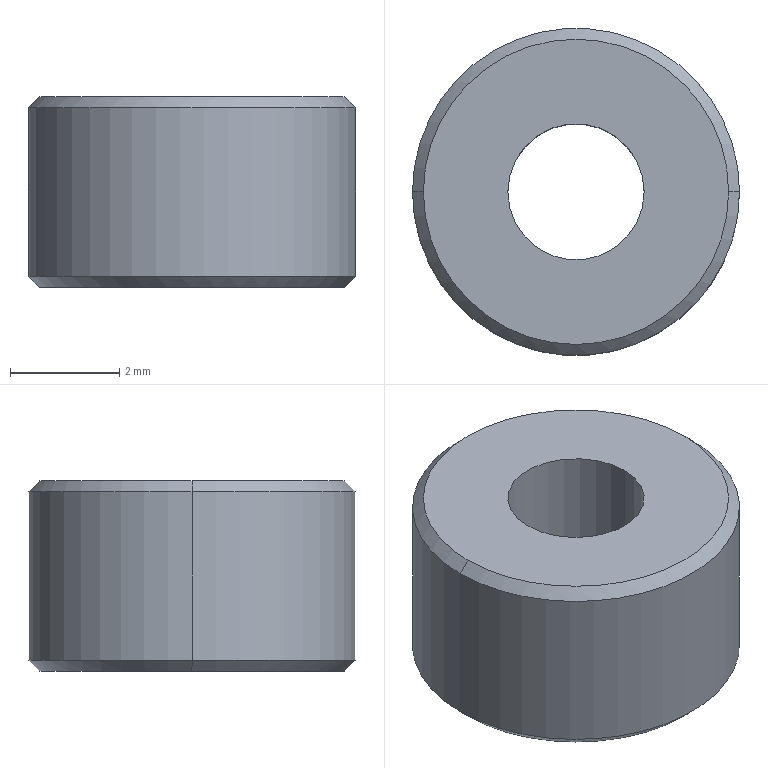Part | SolidWorks | features Chamfer 1, Extrusion 1, HoleWzd 1 | 1 solid | 10 faces | box 6 x 6 x 3.5 mm | volume 81.042 mm3 | cone 4 | cylinder 4 | plane 2 | commonest cylinder face diameters 2.5 x2 6 x2
STEP:
#1=CARTESIAN_POINT('',(2.8,0.,3.5));
#2=VERTEX_POINT('',#1);
#3=CARTESIAN_POINT('',(-2.8,0.,3.5));
#4=VERTEX_POINT('',#3);
#5=CARTESIAN_POINT('',(0.,0.,3.5));
#6=DIRECTION('',(0.,0.,1.));
#7=DIRECTION('',(1.,0.,0.));
#8=AXIS2_PLACEMENT_3D('',#5,#6,#7);
#9=CIRCLE('',#8,2.8);
#10=EDGE_CURVE('',#2,#4,#9,.T.);
#11=ORIENTED_EDGE('',*,*,#10,.F.);
#12=CARTESIAN_POINT('',(3.,0.,3.3));
#13=VERTEX_POINT('',#12);
#14=CARTESIAN_POINT('',(2.8,0.,3.5));
#15=DIRECTION('',(0.7071,0.,-0.7071));
#16=VECTOR('',#15,1000.);
#17=LINE('',#14,#16);
#18=EDGE_CURVE('',#2,#13,#17,.T.);
#19=ORIENTED_EDGE('',*,*,#18,.T.);
#20=CARTESIAN_POINT('',(-3.,0.,3.3));
#21=VERTEX_POINT('',#20);
#22=CARTESIAN_POINT('',(0.,0.,3.3));
#23=DIRECTION('',(0.,0.,-1.));
#24=DIRECTION('',(1.,0.,0.));
#25=AXIS2_PLACEMENT_3D('',#22,#23,#24);
#26=CIRCLE('',#25,3.);
#27=EDGE_CURVE('',#21,#13,#26,.T.);
#28=ORIENTED_EDGE('',*,*,#27,.F.);
#29=CARTESIAN_POINT('',(-2.8,0.,3.5));
#30=DIRECTION('',(-0.7071,0.,-0.7071));
#31=VECTOR('',#30,1000.);
#32=LINE('',#29,#31);
#33=EDGE_CURVE('',#4,#21,#32,.T.);
#34=ORIENTED_EDGE('',*,*,#33,.F.);
#35=EDGE_LOOP('',(#11,#19,#28,#34));
#36=FACE_OUTER_BOUND('',#35,.T.);
#37=CARTESIAN_POINT('',(0.,0.,3.5));
#38=DIRECTION('',(0.,0.,-1.));
#39=DIRECTION('',(-1.,0.,0.));
#40=AXIS2_PLACEMENT_3D('',#37,#38,#39);
#41=CONICAL_SURFACE('',#40,2.8,0.7854);
#42=ADVANCED_FACE('',(#36),#41,.T.);
#43=CARTESIAN_POINT('',(-2.8,0.,0.));
#44=VERTEX_POINT('',#43);
#45=CARTESIAN_POINT('',(2.8,0.,0.));
#46=VERTEX_POINT('',#45);
#47=CARTESIAN_POINT('',(0.,0.,0.));
#48=DIRECTION('',(0.,0.,-1.));
#49=DIRECTION('',(1.,0.,0.));
#50=AXIS2_PLACEMENT_3D('',#47,#48,#49);
#51=CIRCLE('',#50,2.8);
#52=EDGE_CURVE('',#44,#46,#51,.T.);
#53=ORIENTED_EDGE('',*,*,#52,.F.);
#54=CARTESIAN_POINT('',(-3.,0.,0.2));
#55=VERTEX_POINT('',#54);
#56=CARTESIAN_POINT('',(-3.,0.,0.2));
#57=DIRECTION('',(-0.7071,0.,0.7071));
#58=VECTOR('',#57,1000.);
#59=LINE('',#56,#58);
#60=EDGE_CURVE('',#44,#55,#59,.T.);
#61=ORIENTED_EDGE('',*,*,#60,.T.);
#62=CARTESIAN_POINT('',(3.,0.,0.2));
#63=VERTEX_POINT('',#62);
#64=CARTESIAN_POINT('',(0.,0.,0.2));
#65=DIRECTION('',(0.,0.,1.));
#66=DIRECTION('',(1.,0.,0.));
#67=AXIS2_PLACEMENT_3D('',#64,#65,#66);
#68=CIRCLE('',#67,3.);
#69=EDGE_CURVE('',#63,#55,#68,.T.);
#70=ORIENTED_EDGE('',*,*,#69,.F.);
#71=CARTESIAN_POINT('',(3.,0.,0.2));
#72=DIRECTION('',(0.7071,0.,0.7071));
#73=VECTOR('',#72,1000.);
#74=LINE('',#71,#73);
#75=EDGE_CURVE('',#46,#63,#74,.T.);
#76=ORIENTED_EDGE('',*,*,#75,.F.);
#77=EDGE_LOOP('',(#53,#61,#70,#76));
#78=FACE_OUTER_BOUND('',#77,.T.);
#79=CARTESIAN_POINT('',(0.,0.,0.2));
#80=DIRECTION('',(0.,0.,1.));
#81=DIRECTION('',(1.,0.,0.));
#82=AXIS2_PLACEMENT_3D('',#79,#80,#81);
#83=CONICAL_SURFACE('',#82,3.,0.7854);
#84=ADVANCED_FACE('',(#78),#83,.T.);
#85=CARTESIAN_POINT('',(-1.25,0.,3.5));
#86=VERTEX_POINT('',#85);
#87=CARTESIAN_POINT('',(1.25,0.,3.5));
#88=VERTEX_POINT('',#87);
#89=CARTESIAN_POINT('',(0.,0.,3.5));
#90=DIRECTION('',(0.,0.,1.));
#91=DIRECTION('',(1.,0.,0.));
#92=AXIS2_PLACEMENT_3D('',#89,#90,#91);
#93=CIRCLE('',#92,1.25);
#94=EDGE_CURVE('',#86,#88,#93,.T.);
#95=ORIENTED_EDGE('',*,*,#94,.T.);
#96=CARTESIAN_POINT('',(1.25,0.,0.));
#97=VERTEX_POINT('',#96);
#98=CARTESIAN_POINT('',(1.25,0.,0.));
#99=DIRECTION('',(0.,0.,-1.));
#100=VECTOR('',#99,1000.);
#101=LINE('',#98,#100);
#102=EDGE_CURVE('',#88,#97,#101,.T.);
#103=ORIENTED_EDGE('',*,*,#102,.T.);
#104=CARTESIAN_POINT('',(-1.25,0.,0.));
#105=VERTEX_POINT('',#104);
#106=CARTESIAN_POINT('',(0.,0.,0.));
#107=DIRECTION('',(0.,0.,-1.));
#108=DIRECTION('',(-1.,0.,0.));
#109=AXIS2_PLACEMENT_3D('',#106,#107,#108);
#110=CIRCLE('',#109,1.25);
#111=EDGE_CURVE('',#97,#105,#110,.T.);
#112=ORIENTED_EDGE('',*,*,#111,.T.);
#113=CARTESIAN_POINT('',(-1.25,0.,0.));
#114=DIRECTION('',(0.,0.,-1.));
#115=VECTOR('',#114,1000.);
#116=LINE('',#113,#115);
#117=EDGE_CURVE('',#86,#105,#116,.T.);
#118=ORIENTED_EDGE('',*,*,#117,.F.);
#119=EDGE_LOOP('',(#95,#103,#112,#118));
#120=FACE_OUTER_BOUND('',#119,.T.);
#121=CARTESIAN_POINT('',(0.,0.,0.));
#122=DIRECTION('',(0.,0.,-1.));
#123=DIRECTION('',(-1.,0.,0.));
#124=AXIS2_PLACEMENT_3D('',#121,#122,#123);
#125=CYLINDRICAL_SURFACE('',#124,1.25);
#126=ADVANCED_FACE('',(#120),#125,.F.);
#127=ORIENTED_EDGE('',*,*,#27,.T.);
#128=CARTESIAN_POINT('',(3.,0.,3.5));
#129=DIRECTION('',(0.,0.,-1.));
#130=VECTOR('',#129,1000.);
#131=LINE('',#128,#130);
#132=EDGE_CURVE('',#13,#63,#131,.T.);
#133=ORIENTED_EDGE('',*,*,#132,.T.);
#134=ORIENTED_EDGE('',*,*,#69,.T.);
#135=CARTESIAN_POINT('',(-3.,0.,3.5));
#136=DIRECTION('',(0.,0.,-1.));
#137=VECTOR('',#136,1000.);
#138=LINE('',#135,#137);
#139=EDGE_CURVE('',#21,#55,#138,.T.);
#140=ORIENTED_EDGE('',*,*,#139,.F.);
#141=EDGE_LOOP('',(#127,#133,#134,#140));
#142=FACE_OUTER_BOUND('',#141,.T.);
#143=CARTESIAN_POINT('',(0.,0.,3.5));
#144=DIRECTION('',(0.,0.,-1.));
#145=DIRECTION('',(-1.,0.,0.));
#146=AXIS2_PLACEMENT_3D('',#143,#144,#145);
#147=CYLINDRICAL_SURFACE('',#146,3.);
#148=ADVANCED_FACE('',(#142),#147,.T.);
#149=ORIENTED_EDGE('',*,*,#132,.F.);
#150=CARTESIAN_POINT('',(0.,0.,3.3));
#151=DIRECTION('',(0.,0.,-1.));
#152=DIRECTION('',(1.,0.,0.));
#153=AXIS2_PLACEMENT_3D('',#150,#151,#152);
#154=CIRCLE('',#153,3.);
#155=EDGE_CURVE('',#13,#21,#154,.T.);
#156=ORIENTED_EDGE('',*,*,#155,.T.);
#157=ORIENTED_EDGE('',*,*,#139,.T.);
#158=CARTESIAN_POINT('',(0.,0.,0.2));
#159=DIRECTION('',(0.,0.,1.));
#160=DIRECTION('',(1.,0.,0.));
#161=AXIS2_PLACEMENT_3D('',#158,#159,#160);
#162=CIRCLE('',#161,3.);
#163=EDGE_CURVE('',#55,#63,#162,.T.);
#164=ORIENTED_EDGE('',*,*,#163,.T.);
#165=EDGE_LOOP('',(#149,#156,#157,#164));
#166=FACE_OUTER_BOUND('',#165,.T.);
#167=CARTESIAN_POINT('',(0.,0.,3.5));
#168=DIRECTION('',(0.,0.,-1.));
#169=DIRECTION('',(-1.,0.,0.));
#170=AXIS2_PLACEMENT_3D('',#167,#168,#169);
#171=CYLINDRICAL_SURFACE('',#170,3.);
#172=ADVANCED_FACE('',(#166),#171,.T.);
#173=CARTESIAN_POINT('',(0.,0.,3.5));
#174=DIRECTION('',(0.,0.,1.));
#175=DIRECTION('',(1.,0.,0.));
#176=AXIS2_PLACEMENT_3D('',#173,#174,#175);
#177=CIRCLE('',#176,2.8);
#178=EDGE_CURVE('',#4,#2,#177,.T.);
#179=ORIENTED_EDGE('',*,*,#178,.T.);
#180=ORIENTED_EDGE('',*,*,#10,.T.);
#181=EDGE_LOOP('',(#179,#180));
#182=FACE_OUTER_BOUND('',#181,.T.);
#183=ORIENTED_EDGE('',*,*,#94,.F.);
#184=CARTESIAN_POINT('',(0.,0.,3.5));
#185=DIRECTION('',(0.,0.,1.));
#186=DIRECTION('',(1.,0.,0.));
#187=AXIS2_PLACEMENT_3D('',#184,#185,#186);
#188=CIRCLE('',#187,1.25);
#189=EDGE_CURVE('',#88,#86,#188,.T.);
#190=ORIENTED_EDGE('',*,*,#189,.F.);
#191=EDGE_LOOP('',(#183,#190));
#192=FACE_BOUND('',#191,.T.);
#193=CARTESIAN_POINT('',(0.,0.,3.5));
#194=DIRECTION('',(0.,0.,1.));
#195=DIRECTION('',(1.,0.,0.));
#196=AXIS2_PLACEMENT_3D('',#193,#194,#195);
#197=PLANE('',#196);
#198=ADVANCED_FACE('',(#182,#192),#197,.T.);
#199=CARTESIAN_POINT('',(0.,0.,0.));
#200=DIRECTION('',(0.,0.,-1.));
#201=DIRECTION('',(1.,0.,0.));
#202=AXIS2_PLACEMENT_3D('',#199,#200,#201);
#203=CIRCLE('',#202,2.8);
#204=EDGE_CURVE('',#46,#44,#203,.T.);
#205=ORIENTED_EDGE('',*,*,#204,.T.);
#206=ORIENTED_EDGE('',*,*,#52,.T.);
#207=EDGE_LOOP('',(#205,#206));
#208=FACE_OUTER_BOUND('',#207,.T.);
#209=CARTESIAN_POINT('',(0.,0.,0.));
#210=DIRECTION('',(0.,0.,-1.));
#211=DIRECTION('',(-1.,0.,0.));
#212=AXIS2_PLACEMENT_3D('',#209,#210,#211);
#213=CIRCLE('',#212,1.25);
#214=EDGE_CURVE('',#105,#97,#213,.T.);
#215=ORIENTED_EDGE('',*,*,#214,.F.);
#216=ORIENTED_EDGE('',*,*,#111,.F.);
#217=EDGE_LOOP('',(#215,#216));
#218=FACE_BOUND('',#217,.T.);
#219=CARTESIAN_POINT('',(0.,0.,0.));
#220=DIRECTION('',(0.,0.,1.));
#221=DIRECTION('',(1.,0.,0.));
#222=AXIS2_PLACEMENT_3D('',#219,#220,#221);
#223=PLANE('',#222);
#224=ADVANCED_FACE('',(#208,#218),#223,.F.);
#225=ORIENTED_EDGE('',*,*,#102,.F.);
#226=ORIENTED_EDGE('',*,*,#189,.T.);
#227=ORIENTED_EDGE('',*,*,#117,.T.);
#228=ORIENTED_EDGE('',*,*,#214,.T.);
#229=EDGE_LOOP('',(#225,#226,#227,#228));
#230=FACE_OUTER_BOUND('',#229,.T.);
#231=CARTESIAN_POINT('',(0.,0.,0.));
#232=DIRECTION('',(0.,0.,-1.));
#233=DIRECTION('',(-1.,0.,0.));
#234=AXIS2_PLACEMENT_3D('',#231,#232,#233);
#235=CYLINDRICAL_SURFACE('',#234,1.25);
#236=ADVANCED_FACE('',(#230),#235,.F.);
#237=ORIENTED_EDGE('',*,*,#60,.F.);
#238=ORIENTED_EDGE('',*,*,#204,.F.);
#239=ORIENTED_EDGE('',*,*,#75,.T.);
#240=ORIENTED_EDGE('',*,*,#163,.F.);
#241=EDGE_LOOP('',(#237,#238,#239,#240));
#242=FACE_OUTER_BOUND('',#241,.T.);
#243=CARTESIAN_POINT('',(0.,0.,0.2));
#244=DIRECTION('',(0.,0.,1.));
#245=DIRECTION('',(1.,0.,0.));
#246=AXIS2_PLACEMENT_3D('',#243,#244,#245);
#247=CONICAL_SURFACE('',#246,3.,0.7854);
#248=ADVANCED_FACE('',(#242),#247,.T.);
#249=ORIENTED_EDGE('',*,*,#18,.F.);
#250=ORIENTED_EDGE('',*,*,#178,.F.);
#251=ORIENTED_EDGE('',*,*,#33,.T.);
#252=ORIENTED_EDGE('',*,*,#155,.F.);
#253=EDGE_LOOP('',(#249,#250,#251,#252));
#254=FACE_OUTER_BOUND('',#253,.T.);
#255=CARTESIAN_POINT('',(0.,0.,3.5));
#256=DIRECTION('',(0.,0.,-1.));
#257=DIRECTION('',(-1.,0.,0.));
#258=AXIS2_PLACEMENT_3D('',#255,#256,#257);
#259=CONICAL_SURFACE('',#258,2.8,0.7854);
#260=ADVANCED_FACE('',(#254),#259,.T.);
#261=CLOSED_SHELL('',(#42,#84,#126,#148,#172,#198,#224,#236,#248,#260));
#262=MANIFOLD_SOLID_BREP('',#261);
#263=CARTESIAN_POINT('',(0.,0.,0.));
#264=DIRECTION('',(0.,0.,1.));
#265=DIRECTION('',(1.,0.,0.));
#266=AXIS2_PLACEMENT_3D('',#263,#264,#265);
#267=(LENGTH_UNIT()NAMED_UNIT(*)SI_UNIT(.MILLI.,.METRE.));
#268=UNCERTAINTY_MEASURE_WITH_UNIT(LENGTH_MEASURE(0.00001),#267,'','');
#269=(NAMED_UNIT(*)PLANE_ANGLE_UNIT()SI_UNIT($,.RADIAN.));
#270=(NAMED_UNIT(*)SI_UNIT($,.STERADIAN.)SOLID_ANGLE_UNIT());
#271=(GEOMETRIC_REPRESENTATION_CONTEXT(3)GLOBAL_UNCERTAINTY_ASSIGNED_CONTEXT((#268))GLOBAL_UNIT_ASSIGNED_CONTEXT((#267,#269,#270))REPRESENTATION_CONTEXT('',''));
#272=ADVANCED_BREP_SHAPE_REPRESENTATION('',(#262,#266),#271);